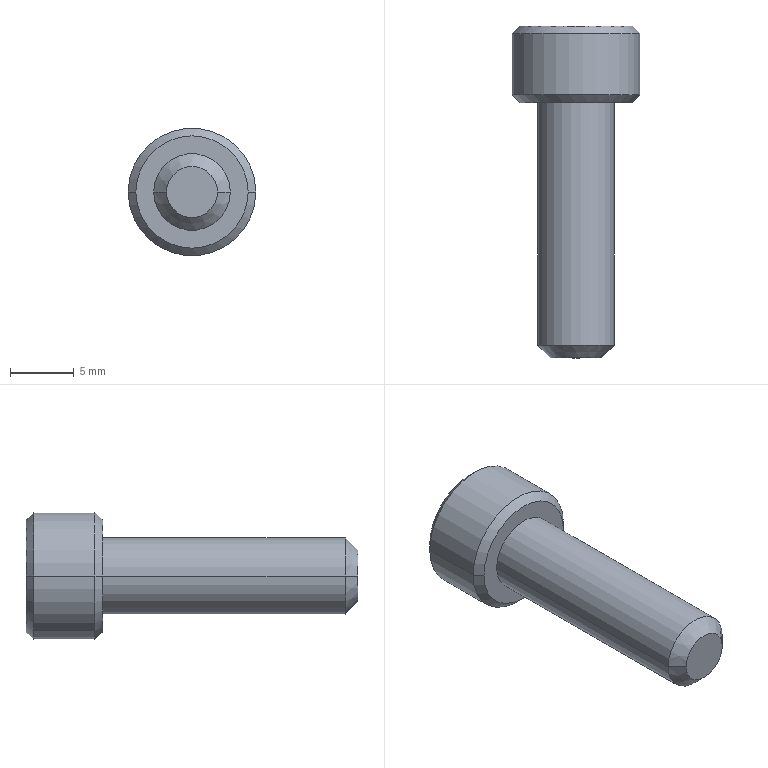Part | STEP file | BB62-M6-20L | 1 solid | 27 faces | box 10 x 26 x 10 mm | volume 939.593 mm3 | plane 15 | cone 8 | cylinder 4 | commonest cylinder face diameters 6 x2 10 x2
STEP:
#1=CARTESIAN_POINT('',(0.,1.349,0.));
#2=VERTEX_POINT('',#1);
#3=CARTESIAN_POINT('',(2.86,3.,0.));
#4=VERTEX_POINT('',#3);
#5=CARTESIAN_POINT('',(0.,1.349,0.));
#6=DIRECTION('',(0.866,0.5,0.));
#7=VECTOR('',#6,1000.);
#8=LINE('',#5,#7);
#9=EDGE_CURVE('',#2,#4,#8,.T.);
#10=ORIENTED_EDGE('',*,*,#9,.F.);
#11=CARTESIAN_POINT('',(-2.86,3.,0.));
#12=VERTEX_POINT('',#11);
#13=CARTESIAN_POINT('',(0.,1.349,0.));
#14=DIRECTION('',(-0.866,0.5,0.));
#15=VECTOR('',#14,1000.);
#16=LINE('',#13,#15);
#17=EDGE_CURVE('',#2,#12,#16,.T.);
#18=ORIENTED_EDGE('',*,*,#17,.T.);
#19=CARTESIAN_POINT('',(-2.477,3.,1.43));
#20=VERTEX_POINT('',#19);
#21=CARTESIAN_POINT('',(0.,3.,0.));
#22=DIRECTION('',(0.,-1.,0.));
#23=DIRECTION('',(-1.,0.,0.));
#24=AXIS2_PLACEMENT_3D('',#21,#22,#23);
#25=CIRCLE('',#24,2.86);
#26=EDGE_CURVE('',#20,#12,#25,.T.);
#27=ORIENTED_EDGE('',*,*,#26,.F.);
#28=CARTESIAN_POINT('',(0.,3.,2.86));
#29=VERTEX_POINT('',#28);
#30=CARTESIAN_POINT('',(0.,3.,0.));
#31=DIRECTION('',(0.,-1.,0.));
#32=DIRECTION('',(-1.,0.,0.));
#33=AXIS2_PLACEMENT_3D('',#30,#31,#32);
#34=CIRCLE('',#33,2.86);
#35=EDGE_CURVE('',#29,#20,#34,.T.);
#36=ORIENTED_EDGE('',*,*,#35,.F.);
#37=CARTESIAN_POINT('',(2.477,3.,1.43));
#38=VERTEX_POINT('',#37);
#39=CARTESIAN_POINT('',(0.,3.,0.));
#40=DIRECTION('',(0.,-1.,0.));
#41=DIRECTION('',(-1.,0.,0.));
#42=AXIS2_PLACEMENT_3D('',#39,#40,#41);
#43=CIRCLE('',#42,2.86);
#44=EDGE_CURVE('',#38,#29,#43,.T.);
#45=ORIENTED_EDGE('',*,*,#44,.F.);
#46=CARTESIAN_POINT('',(0.,3.,0.));
#47=DIRECTION('',(0.,-1.,0.));
#48=DIRECTION('',(-1.,0.,0.));
#49=AXIS2_PLACEMENT_3D('',#46,#47,#48);
#50=CIRCLE('',#49,2.86);
#51=EDGE_CURVE('',#4,#38,#50,.T.);
#52=ORIENTED_EDGE('',*,*,#51,.F.);
#53=EDGE_LOOP('',(#10,#18,#27,#36,#45,#52));
#54=FACE_OUTER_BOUND('',#53,.T.);
#55=CARTESIAN_POINT('',(0.,1001.349,0.));
#56=DIRECTION('',(0.,1.,0.));
#57=DIRECTION('',(1.,0.,0.));
#58=AXIS2_PLACEMENT_3D('',#55,#56,#57);
#59=CONICAL_SURFACE('',#58,1732.051,1.047);
#60=ADVANCED_FACE('',(#54),#59,.F.);
#61=CARTESIAN_POINT('',(2.,-20.,0.));
#62=VERTEX_POINT('',#61);
#63=CARTESIAN_POINT('',(-2.,-20.,0.));
#64=VERTEX_POINT('',#63);
#65=CARTESIAN_POINT('',(0.,-20.,0.));
#66=DIRECTION('',(0.,1.,0.));
#67=DIRECTION('',(1.,0.,0.));
#68=AXIS2_PLACEMENT_3D('',#65,#66,#67);
#69=CIRCLE('',#68,2.);
#70=EDGE_CURVE('',#62,#64,#69,.T.);
#71=ORIENTED_EDGE('',*,*,#70,.T.);
#72=CARTESIAN_POINT('',(-3.,-19.,0.));
#73=VERTEX_POINT('',#72);
#74=CARTESIAN_POINT('',(-2.,-20.,0.));
#75=DIRECTION('',(-0.7071,0.7071,0.));
#76=VECTOR('',#75,1000.);
#77=LINE('',#74,#76);
#78=EDGE_CURVE('',#64,#73,#77,.T.);
#79=ORIENTED_EDGE('',*,*,#78,.T.);
#80=CARTESIAN_POINT('',(3.,-19.,0.));
#81=VERTEX_POINT('',#80);
#82=CARTESIAN_POINT('',(0.,-19.,0.));
#83=DIRECTION('',(0.,-1.,0.));
#84=DIRECTION('',(-1.,0.,0.));
#85=AXIS2_PLACEMENT_3D('',#82,#83,#84);
#86=CIRCLE('',#85,3.);
#87=EDGE_CURVE('',#73,#81,#86,.T.);
#88=ORIENTED_EDGE('',*,*,#87,.T.);
#89=CARTESIAN_POINT('',(2.,-20.,0.));
#90=DIRECTION('',(0.7071,0.7071,0.));
#91=VECTOR('',#90,1000.);
#92=LINE('',#89,#91);
#93=EDGE_CURVE('',#62,#81,#92,.T.);
#94=ORIENTED_EDGE('',*,*,#93,.F.);
#95=EDGE_LOOP('',(#71,#79,#88,#94));
#96=FACE_OUTER_BOUND('',#95,.T.);
#97=CARTESIAN_POINT('',(0.,-20.,0.));
#98=DIRECTION('',(0.,1.,0.));
#99=DIRECTION('',(1.,0.,0.));
#100=AXIS2_PLACEMENT_3D('',#97,#98,#99);
#101=CONICAL_SURFACE('',#100,2.,0.7854);
#102=ADVANCED_FACE('',(#96),#101,.T.);
#103=ORIENTED_EDGE('',*,*,#87,.F.);
#104=CARTESIAN_POINT('',(-3.,0.,0.));
#105=VERTEX_POINT('',#104);
#106=CARTESIAN_POINT('',(-3.,-19.,0.));
#107=DIRECTION('',(0.,1.,0.));
#108=VECTOR('',#107,1000.);
#109=LINE('',#106,#108);
#110=EDGE_CURVE('',#73,#105,#109,.T.);
#111=ORIENTED_EDGE('',*,*,#110,.T.);
#112=CARTESIAN_POINT('',(3.,0.,0.));
#113=VERTEX_POINT('',#112);
#114=CARTESIAN_POINT('',(0.,0.,0.));
#115=DIRECTION('',(0.,-1.,0.));
#116=DIRECTION('',(-1.,0.,0.));
#117=AXIS2_PLACEMENT_3D('',#114,#115,#116);
#118=CIRCLE('',#117,3.);
#119=EDGE_CURVE('',#105,#113,#118,.T.);
#120=ORIENTED_EDGE('',*,*,#119,.T.);
#121=CARTESIAN_POINT('',(3.,-19.,0.));
#122=DIRECTION('',(0.,1.,0.));
#123=VECTOR('',#122,1000.);
#124=LINE('',#121,#123);
#125=EDGE_CURVE('',#81,#113,#124,.T.);
#126=ORIENTED_EDGE('',*,*,#125,.F.);
#127=EDGE_LOOP('',(#103,#111,#120,#126));
#128=FACE_OUTER_BOUND('',#127,.T.);
#129=CARTESIAN_POINT('',(0.,-19.,0.));
#130=DIRECTION('',(0.,1.,0.));
#131=DIRECTION('',(1.,0.,0.));
#132=AXIS2_PLACEMENT_3D('',#129,#130,#131);
#133=CYLINDRICAL_SURFACE('',#132,3.);
#134=ADVANCED_FACE('',(#128),#133,.T.);
#135=CARTESIAN_POINT('',(-4.4,6.,0.));
#136=VERTEX_POINT('',#135);
#137=CARTESIAN_POINT('',(4.4,6.,0.));
#138=VERTEX_POINT('',#137);
#139=CARTESIAN_POINT('',(0.,6.,0.));
#140=DIRECTION('',(0.,-1.,0.));
#141=DIRECTION('',(-1.,0.,0.));
#142=AXIS2_PLACEMENT_3D('',#139,#140,#141);
#143=CIRCLE('',#142,4.4);
#144=EDGE_CURVE('',#136,#138,#143,.T.);
#145=ORIENTED_EDGE('',*,*,#144,.T.);
#146=CARTESIAN_POINT('',(5.,5.4,0.));
#147=VERTEX_POINT('',#146);
#148=CARTESIAN_POINT('',(5.,5.4,0.));
#149=DIRECTION('',(0.7071,-0.7071,0.));
#150=VECTOR('',#149,1000.);
#151=LINE('',#148,#150);
#152=EDGE_CURVE('',#138,#147,#151,.T.);
#153=ORIENTED_EDGE('',*,*,#152,.T.);
#154=CARTESIAN_POINT('',(-5.,5.4,0.));
#155=VERTEX_POINT('',#154);
#156=CARTESIAN_POINT('',(0.,5.4,0.));
#157=DIRECTION('',(0.,-1.,0.));
#158=DIRECTION('',(-1.,0.,0.));
#159=AXIS2_PLACEMENT_3D('',#156,#157,#158);
#160=CIRCLE('',#159,5.);
#161=EDGE_CURVE('',#155,#147,#160,.T.);
#162=ORIENTED_EDGE('',*,*,#161,.F.);
#163=CARTESIAN_POINT('',(-5.,5.4,0.));
#164=DIRECTION('',(-0.7071,-0.7071,0.));
#165=VECTOR('',#164,1000.);
#166=LINE('',#163,#165);
#167=EDGE_CURVE('',#136,#155,#166,.T.);
#168=ORIENTED_EDGE('',*,*,#167,.F.);
#169=EDGE_LOOP('',(#145,#153,#162,#168));
#170=FACE_OUTER_BOUND('',#169,.T.);
#171=CARTESIAN_POINT('',(0.,5.4,0.));
#172=DIRECTION('',(0.,-1.,0.));
#173=DIRECTION('',(-1.,0.,0.));
#174=AXIS2_PLACEMENT_3D('',#171,#172,#173);
#175=CONICAL_SURFACE('',#174,5.,0.7854);
#176=ADVANCED_FACE('',(#170),#175,.T.);
#177=ORIENTED_EDGE('',*,*,#161,.T.);
#178=CARTESIAN_POINT('',(5.,0.6,0.));
#179=VERTEX_POINT('',#178);
#180=CARTESIAN_POINT('',(5.,1.62,0.));
#181=DIRECTION('',(0.,-1.,0.));
#182=VECTOR('',#181,1000.);
#183=LINE('',#180,#182);
#184=EDGE_CURVE('',#147,#179,#183,.T.);
#185=ORIENTED_EDGE('',*,*,#184,.T.);
#186=CARTESIAN_POINT('',(-5.,0.6,0.));
#187=VERTEX_POINT('',#186);
#188=CARTESIAN_POINT('',(0.,0.6,0.));
#189=DIRECTION('',(0.,-1.,0.));
#190=DIRECTION('',(-1.,0.,0.));
#191=AXIS2_PLACEMENT_3D('',#188,#189,#190);
#192=CIRCLE('',#191,5.);
#193=EDGE_CURVE('',#187,#179,#192,.T.);
#194=ORIENTED_EDGE('',*,*,#193,.F.);
#195=CARTESIAN_POINT('',(-5.,1.62,0.));
#196=DIRECTION('',(0.,-1.,0.));
#197=VECTOR('',#196,1000.);
#198=LINE('',#195,#197);
#199=EDGE_CURVE('',#155,#187,#198,.T.);
#200=ORIENTED_EDGE('',*,*,#199,.F.);
#201=EDGE_LOOP('',(#177,#185,#194,#200));
#202=FACE_OUTER_BOUND('',#201,.T.);
#203=CARTESIAN_POINT('',(0.,1.62,0.));
#204=DIRECTION('',(0.,-1.,0.));
#205=DIRECTION('',(-1.,0.,0.));
#206=AXIS2_PLACEMENT_3D('',#203,#204,#205);
#207=CYLINDRICAL_SURFACE('',#206,5.);
#208=ADVANCED_FACE('',(#202),#207,.T.);
#209=CARTESIAN_POINT('',(-4.4,0.,0.));
#210=VERTEX_POINT('',#209);
#211=CARTESIAN_POINT('',(4.4,0.,0.));
#212=VERTEX_POINT('',#211);
#213=CARTESIAN_POINT('',(0.,0.,0.));
#214=DIRECTION('',(0.,-1.,0.));
#215=DIRECTION('',(-1.,0.,0.));
#216=AXIS2_PLACEMENT_3D('',#213,#214,#215);
#217=CIRCLE('',#216,4.4);
#218=EDGE_CURVE('',#210,#212,#217,.T.);
#219=ORIENTED_EDGE('',*,*,#218,.F.);
#220=CARTESIAN_POINT('',(-4.4,0.,0.));
#221=DIRECTION('',(-0.7071,0.7071,0.));
#222=VECTOR('',#221,1000.);
#223=LINE('',#220,#222);
#224=EDGE_CURVE('',#210,#187,#223,.T.);
#225=ORIENTED_EDGE('',*,*,#224,.T.);
#226=ORIENTED_EDGE('',*,*,#193,.T.);
#227=CARTESIAN_POINT('',(4.4,0.,0.));
#228=DIRECTION('',(0.7071,0.7071,0.));
#229=VECTOR('',#228,1000.);
#230=LINE('',#227,#229);
#231=EDGE_CURVE('',#212,#179,#230,.T.);
#232=ORIENTED_EDGE('',*,*,#231,.F.);
#233=EDGE_LOOP('',(#219,#225,#226,#232));
#234=FACE_OUTER_BOUND('',#233,.T.);
#235=CARTESIAN_POINT('',(0.,0.,0.));
#236=DIRECTION('',(0.,1.,0.));
#237=DIRECTION('',(1.,0.,0.));
#238=AXIS2_PLACEMENT_3D('',#235,#236,#237);
#239=CONICAL_SURFACE('',#238,4.4,0.7854);
#240=ADVANCED_FACE('',(#234),#239,.T.);
#241=ORIENTED_EDGE('',*,*,#144,.F.);
#242=CARTESIAN_POINT('',(0.,6.,0.));
#243=DIRECTION('',(0.,-1.,0.));
#244=DIRECTION('',(-1.,0.,0.));
#245=AXIS2_PLACEMENT_3D('',#242,#243,#244);
#246=CIRCLE('',#245,4.4);
#247=EDGE_CURVE('',#138,#136,#246,.T.);
#248=ORIENTED_EDGE('',*,*,#247,.F.);
#249=EDGE_LOOP('',(#241,#248));
#250=FACE_OUTER_BOUND('',#249,.T.);
#251=CARTESIAN_POINT('',(0.,6.,-2.86));
#252=VERTEX_POINT('',#251);
#253=CARTESIAN_POINT('',(-2.477,6.,-1.43));
#254=VERTEX_POINT('',#253);
#255=CARTESIAN_POINT('',(0.,6.,-2.86));
#256=DIRECTION('',(-0.866,0.,0.5));
#257=VECTOR('',#256,1000.);
#258=LINE('',#255,#257);
#259=EDGE_CURVE('',#252,#254,#258,.T.);
#260=ORIENTED_EDGE('',*,*,#259,.F.);
#261=CARTESIAN_POINT('',(2.477,6.,-1.43));
#262=VERTEX_POINT('',#261);
#263=CARTESIAN_POINT('',(2.477,6.,-1.43));
#264=DIRECTION('',(-0.866,0.,-0.5));
#265=VECTOR('',#264,1000.);
#266=LINE('',#263,#265);
#267=EDGE_CURVE('',#262,#252,#266,.T.);
#268=ORIENTED_EDGE('',*,*,#267,.F.);
#269=CARTESIAN_POINT('',(2.477,6.,1.43));
#270=VERTEX_POINT('',#269);
#271=CARTESIAN_POINT('',(2.477,6.,1.43));
#272=DIRECTION('',(0.,0.,-1.));
#273=VECTOR('',#272,1000.);
#274=LINE('',#271,#273);
#275=EDGE_CURVE('',#270,#262,#274,.T.);
#276=ORIENTED_EDGE('',*,*,#275,.F.);
#277=CARTESIAN_POINT('',(0.,6.,2.86));
#278=VERTEX_POINT('',#277);
#279=CARTESIAN_POINT('',(0.,6.,2.86));
#280=DIRECTION('',(0.866,0.,-0.5));
#281=VECTOR('',#280,1000.);
#282=LINE('',#279,#281);
#283=EDGE_CURVE('',#278,#270,#282,.T.);
#284=ORIENTED_EDGE('',*,*,#283,.F.);
#285=CARTESIAN_POINT('',(-2.477,6.,1.43));
#286=VERTEX_POINT('',#285);
#287=CARTESIAN_POINT('',(-2.477,6.,1.43));
#288=DIRECTION('',(0.866,0.,0.5));
#289=VECTOR('',#288,1000.);
#290=LINE('',#287,#289);
#291=EDGE_CURVE('',#286,#278,#290,.T.);
#292=ORIENTED_EDGE('',*,*,#291,.F.);
#293=CARTESIAN_POINT('',(-2.477,6.,-1.43));
#294=DIRECTION('',(0.,0.,1.));
#295=VECTOR('',#294,1000.);
#296=LINE('',#293,#295);
#297=EDGE_CURVE('',#254,#286,#296,.T.);
#298=ORIENTED_EDGE('',*,*,#297,.F.);
#299=EDGE_LOOP('',(#260,#268,#276,#284,#292,#298));
#300=FACE_BOUND('',#299,.T.);
#301=CARTESIAN_POINT('',(4.4,6.,0.));
#302=DIRECTION('',(0.,1.,0.));
#303=DIRECTION('',(1.,0.,0.));
#304=AXIS2_PLACEMENT_3D('',#301,#302,#303);
#305=PLANE('',#304);
#306=ADVANCED_FACE('',(#250,#300),#305,.T.);
#307=CARTESIAN_POINT('',(0.,0.,0.));
#308=DIRECTION('',(0.,-1.,0.));
#309=DIRECTION('',(-1.,0.,0.));
#310=AXIS2_PLACEMENT_3D('',#307,#308,#309);
#311=CIRCLE('',#310,3.);
#312=EDGE_CURVE('',#113,#105,#311,.T.);
#313=ORIENTED_EDGE('',*,*,#312,.F.);
#314=ORIENTED_EDGE('',*,*,#119,.F.);
#315=EDGE_LOOP('',(#313,#314));
#316=FACE_BOUND('',#315,.T.);
#317=CARTESIAN_POINT('',(0.,0.,0.));
#318=DIRECTION('',(0.,-1.,0.));
#319=DIRECTION('',(-1.,0.,0.));
#320=AXIS2_PLACEMENT_3D('',#317,#318,#319);
#321=CIRCLE('',#320,4.4);
#322=EDGE_CURVE('',#212,#210,#321,.T.);
#323=ORIENTED_EDGE('',*,*,#322,.T.);
#324=ORIENTED_EDGE('',*,*,#218,.T.);
#325=EDGE_LOOP('',(#323,#324));
#326=FACE_OUTER_BOUND('',#325,.T.);
#327=CARTESIAN_POINT('',(0.,0.,0.));
#328=DIRECTION('',(0.,-1.,0.));
#329=DIRECTION('',(-1.,0.,0.));
#330=AXIS2_PLACEMENT_3D('',#327,#328,#329);
#331=PLANE('',#330);
#332=ADVANCED_FACE('',(#316,#326),#331,.T.);
#333=ORIENTED_EDGE('',*,*,#224,.F.);
#334=ORIENTED_EDGE('',*,*,#322,.F.);
#335=ORIENTED_EDGE('',*,*,#231,.T.);
#336=CARTESIAN_POINT('',(0.,0.6,0.));
#337=DIRECTION('',(0.,-1.,0.));
#338=DIRECTION('',(-1.,0.,0.));
#339=AXIS2_PLACEMENT_3D('',#336,#337,#338);
#340=CIRCLE('',#339,5.);
#341=EDGE_CURVE('',#179,#187,#340,.T.);
#342=ORIENTED_EDGE('',*,*,#341,.T.);
#343=EDGE_LOOP('',(#333,#334,#335,#342));
#344=FACE_OUTER_BOUND('',#343,.T.);
#345=CARTESIAN_POINT('',(0.,0.,0.));
#346=DIRECTION('',(0.,1.,0.));
#347=DIRECTION('',(1.,0.,0.));
#348=AXIS2_PLACEMENT_3D('',#345,#346,#347);
#349=CONICAL_SURFACE('',#348,4.4,0.7854);
#350=ADVANCED_FACE('',(#344),#349,.T.);
#351=ORIENTED_EDGE('',*,*,#184,.F.);
#352=CARTESIAN_POINT('',(0.,5.4,0.));
#353=DIRECTION('',(0.,-1.,0.));
#354=DIRECTION('',(-1.,0.,0.));
#355=AXIS2_PLACEMENT_3D('',#352,#353,#354);
#356=CIRCLE('',#355,5.);
#357=EDGE_CURVE('',#147,#155,#356,.T.);
#358=ORIENTED_EDGE('',*,*,#357,.T.);
#359=ORIENTED_EDGE('',*,*,#199,.T.);
#360=ORIENTED_EDGE('',*,*,#341,.F.);
#361=EDGE_LOOP('',(#351,#358,#359,#360));
#362=FACE_OUTER_BOUND('',#361,.T.);
#363=CARTESIAN_POINT('',(0.,1.62,0.));
#364=DIRECTION('',(0.,-1.,0.));
#365=DIRECTION('',(-1.,0.,0.));
#366=AXIS2_PLACEMENT_3D('',#363,#364,#365);
#367=CYLINDRICAL_SURFACE('',#366,5.);
#368=ADVANCED_FACE('',(#362),#367,.T.);
#369=ORIENTED_EDGE('',*,*,#152,.F.);
#370=ORIENTED_EDGE('',*,*,#247,.T.);
#371=ORIENTED_EDGE('',*,*,#167,.T.);
#372=ORIENTED_EDGE('',*,*,#357,.F.);
#373=EDGE_LOOP('',(#369,#370,#371,#372));
#374=FACE_OUTER_BOUND('',#373,.T.);
#375=CARTESIAN_POINT('',(0.,5.4,0.));
#376=DIRECTION('',(0.,-1.,0.));
#377=DIRECTION('',(-1.,0.,0.));
#378=AXIS2_PLACEMENT_3D('',#375,#376,#377);
#379=CONICAL_SURFACE('',#378,5.,0.7854);
#380=ADVANCED_FACE('',(#374),#379,.T.);
#381=ORIENTED_EDGE('',*,*,#110,.F.);
#382=CARTESIAN_POINT('',(0.,-19.,0.));
#383=DIRECTION('',(0.,-1.,0.));
#384=DIRECTION('',(-1.,0.,0.));
#385=AXIS2_PLACEMENT_3D('',#382,#383,#384);
#386=CIRCLE('',#385,3.);
#387=EDGE_CURVE('',#81,#73,#386,.T.);
#388=ORIENTED_EDGE('',*,*,#387,.F.);
#389=ORIENTED_EDGE('',*,*,#125,.T.);
#390=ORIENTED_EDGE('',*,*,#312,.T.);
#391=EDGE_LOOP('',(#381,#388,#389,#390));
#392=FACE_OUTER_BOUND('',#391,.T.);
#393=CARTESIAN_POINT('',(0.,-19.,0.));
#394=DIRECTION('',(0.,1.,0.));
#395=DIRECTION('',(1.,0.,0.));
#396=AXIS2_PLACEMENT_3D('',#393,#394,#395);
#397=CYLINDRICAL_SURFACE('',#396,3.);
#398=ADVANCED_FACE('',(#392),#397,.T.);
#399=ORIENTED_EDGE('',*,*,#70,.F.);
#400=CARTESIAN_POINT('',(0.,-20.,0.));
#401=DIRECTION('',(0.,1.,0.));
#402=DIRECTION('',(1.,0.,0.));
#403=AXIS2_PLACEMENT_3D('',#400,#401,#402);
#404=CIRCLE('',#403,2.);
#405=EDGE_CURVE('',#64,#62,#404,.T.);
#406=ORIENTED_EDGE('',*,*,#405,.F.);
#407=EDGE_LOOP('',(#399,#406));
#408=FACE_OUTER_BOUND('',#407,.T.);
#409=CARTESIAN_POINT('',(0.,-20.,0.));
#410=DIRECTION('',(0.,-1.,0.));
#411=DIRECTION('',(-1.,0.,0.));
#412=AXIS2_PLACEMENT_3D('',#409,#410,#411);
#413=PLANE('',#412);
#414=ADVANCED_FACE('',(#408),#413,.T.);
#415=ORIENTED_EDGE('',*,*,#78,.F.);
#416=ORIENTED_EDGE('',*,*,#405,.T.);
#417=ORIENTED_EDGE('',*,*,#93,.T.);
#418=ORIENTED_EDGE('',*,*,#387,.T.);
#419=EDGE_LOOP('',(#415,#416,#417,#418));
#420=FACE_OUTER_BOUND('',#419,.T.);
#421=CARTESIAN_POINT('',(0.,-20.,0.));
#422=DIRECTION('',(0.,1.,0.));
#423=DIRECTION('',(1.,0.,0.));
#424=AXIS2_PLACEMENT_3D('',#421,#422,#423);
#425=CONICAL_SURFACE('',#424,2.,0.7854);
#426=ADVANCED_FACE('',(#420),#425,.T.);
#427=CARTESIAN_POINT('',(2.477,3.,-1.43));
#428=VERTEX_POINT('',#427);
#429=CARTESIAN_POINT('',(0.,3.,-2.86));
#430=VERTEX_POINT('',#429);
#431=CARTESIAN_POINT('',(2.477,3.,-1.43));
#432=DIRECTION('',(-0.866,0.,-0.5));
#433=VECTOR('',#432,1000.);
#434=LINE('',#431,#433);
#435=EDGE_CURVE('',#428,#430,#434,.T.);
#436=ORIENTED_EDGE('',*,*,#435,.F.);
#437=CARTESIAN_POINT('',(2.477,6.,-1.43));
#438=DIRECTION('',(0.,-1.,0.));
#439=VECTOR('',#438,1000.);
#440=LINE('',#437,#439);
#441=EDGE_CURVE('',#262,#428,#440,.T.);
#442=ORIENTED_EDGE('',*,*,#441,.F.);
#443=ORIENTED_EDGE('',*,*,#267,.T.);
#444=CARTESIAN_POINT('',(0.,6.,-2.86));
#445=DIRECTION('',(0.,-1.,0.));
#446=VECTOR('',#445,1000.);
#447=LINE('',#444,#446);
#448=EDGE_CURVE('',#252,#430,#447,.T.);
#449=ORIENTED_EDGE('',*,*,#448,.T.);
#450=EDGE_LOOP('',(#436,#442,#443,#449));
#451=FACE_OUTER_BOUND('',#450,.T.);
#452=CARTESIAN_POINT('',(2.477,6.,-1.43));
#453=DIRECTION('',(-0.5,0.,0.866));
#454=DIRECTION('',(0.866,0.,0.5));
#455=AXIS2_PLACEMENT_3D('',#452,#453,#454);
#456=PLANE('',#455);
#457=ADVANCED_FACE('',(#451),#456,.T.);
#458=CARTESIAN_POINT('',(-2.477,3.,-1.43));
#459=VERTEX_POINT('',#458);
#460=CARTESIAN_POINT('',(0.,3.,-2.86));
#461=DIRECTION('',(-0.866,0.,0.5));
#462=VECTOR('',#461,1000.);
#463=LINE('',#460,#462);
#464=EDGE_CURVE('',#430,#459,#463,.T.);
#465=ORIENTED_EDGE('',*,*,#464,.F.);
#466=ORIENTED_EDGE('',*,*,#448,.F.);
#467=ORIENTED_EDGE('',*,*,#259,.T.);
#468=CARTESIAN_POINT('',(-2.477,6.,-1.43));
#469=DIRECTION('',(0.,-1.,0.));
#470=VECTOR('',#469,1000.);
#471=LINE('',#468,#470);
#472=EDGE_CURVE('',#254,#459,#471,.T.);
#473=ORIENTED_EDGE('',*,*,#472,.T.);
#474=EDGE_LOOP('',(#465,#466,#467,#473));
#475=FACE_OUTER_BOUND('',#474,.T.);
#476=CARTESIAN_POINT('',(0.,6.,-2.86));
#477=DIRECTION('',(0.5,0.,0.866));
#478=DIRECTION('',(0.866,0.,-0.5));
#479=AXIS2_PLACEMENT_3D('',#476,#477,#478);
#480=PLANE('',#479);
#481=ADVANCED_FACE('',(#475),#480,.T.);
#482=CARTESIAN_POINT('',(-2.477,3.,-1.43));
#483=DIRECTION('',(0.,0.,1.));
#484=VECTOR('',#483,1000.);
#485=LINE('',#482,#484);
#486=EDGE_CURVE('',#459,#20,#485,.T.);
#487=ORIENTED_EDGE('',*,*,#486,.F.);
#488=ORIENTED_EDGE('',*,*,#472,.F.);
#489=ORIENTED_EDGE('',*,*,#297,.T.);
#490=CARTESIAN_POINT('',(-2.477,6.,1.43));
#491=DIRECTION('',(0.,-1.,0.));
#492=VECTOR('',#491,1000.);
#493=LINE('',#490,#492);
#494=EDGE_CURVE('',#286,#20,#493,.T.);
#495=ORIENTED_EDGE('',*,*,#494,.T.);
#496=EDGE_LOOP('',(#487,#488,#489,#495));
#497=FACE_OUTER_BOUND('',#496,.T.);
#498=CARTESIAN_POINT('',(-2.477,6.,-1.43));
#499=DIRECTION('',(1.,0.,0.));
#500=DIRECTION('',(0.,0.,-1.));
#501=AXIS2_PLACEMENT_3D('',#498,#499,#500);
#502=PLANE('',#501);
#503=ADVANCED_FACE('',(#497),#502,.T.);
#504=CARTESIAN_POINT('',(-2.477,3.,1.43));
#505=DIRECTION('',(0.866,0.,0.5));
#506=VECTOR('',#505,1000.);
#507=LINE('',#504,#506);
#508=EDGE_CURVE('',#20,#29,#507,.T.);
#509=ORIENTED_EDGE('',*,*,#508,.F.);
#510=ORIENTED_EDGE('',*,*,#494,.F.);
#511=ORIENTED_EDGE('',*,*,#291,.T.);
#512=CARTESIAN_POINT('',(0.,6.,2.86));
#513=DIRECTION('',(0.,-1.,0.));
#514=VECTOR('',#513,1000.);
#515=LINE('',#512,#514);
#516=EDGE_CURVE('',#278,#29,#515,.T.);
#517=ORIENTED_EDGE('',*,*,#516,.T.);
#518=EDGE_LOOP('',(#509,#510,#511,#517));
#519=FACE_OUTER_BOUND('',#518,.T.);
#520=CARTESIAN_POINT('',(-2.477,6.,1.43));
#521=DIRECTION('',(0.5,0.,-0.866));
#522=DIRECTION('',(-0.866,0.,-0.5));
#523=AXIS2_PLACEMENT_3D('',#520,#521,#522);
#524=PLANE('',#523);
#525=ADVANCED_FACE('',(#519),#524,.T.);
#526=CARTESIAN_POINT('',(0.,3.,2.86));
#527=DIRECTION('',(0.866,0.,-0.5));
#528=VECTOR('',#527,1000.);
#529=LINE('',#526,#528);
#530=EDGE_CURVE('',#29,#38,#529,.T.);
#531=ORIENTED_EDGE('',*,*,#530,.F.);
#532=ORIENTED_EDGE('',*,*,#516,.F.);
#533=ORIENTED_EDGE('',*,*,#283,.T.);
#534=CARTESIAN_POINT('',(2.477,6.,1.43));
#535=DIRECTION('',(0.,-1.,0.));
#536=VECTOR('',#535,1000.);
#537=LINE('',#534,#536);
#538=EDGE_CURVE('',#270,#38,#537,.T.);
#539=ORIENTED_EDGE('',*,*,#538,.T.);
#540=EDGE_LOOP('',(#531,#532,#533,#539));
#541=FACE_OUTER_BOUND('',#540,.T.);
#542=CARTESIAN_POINT('',(0.,6.,2.86));
#543=DIRECTION('',(-0.5,0.,-0.866));
#544=DIRECTION('',(-0.866,0.,0.5));
#545=AXIS2_PLACEMENT_3D('',#542,#543,#544);
#546=PLANE('',#545);
#547=ADVANCED_FACE('',(#541),#546,.T.);
#548=CARTESIAN_POINT('',(2.477,3.,1.43));
#549=DIRECTION('',(0.,0.,-1.));
#550=VECTOR('',#549,1000.);
#551=LINE('',#548,#550);
#552=EDGE_CURVE('',#38,#428,#551,.T.);
#553=ORIENTED_EDGE('',*,*,#552,.F.);
#554=ORIENTED_EDGE('',*,*,#538,.F.);
#555=ORIENTED_EDGE('',*,*,#275,.T.);
#556=ORIENTED_EDGE('',*,*,#441,.T.);
#557=EDGE_LOOP('',(#553,#554,#555,#556));
#558=FACE_OUTER_BOUND('',#557,.T.);
#559=CARTESIAN_POINT('',(2.477,6.,1.43));
#560=DIRECTION('',(-1.,0.,0.));
#561=DIRECTION('',(0.,0.,1.));
#562=AXIS2_PLACEMENT_3D('',#559,#560,#561);
#563=PLANE('',#562);
#564=ADVANCED_FACE('',(#558),#563,.T.);
#565=ORIENTED_EDGE('',*,*,#435,.T.);
#566=CARTESIAN_POINT('',(0.,3.,0.));
#567=DIRECTION('',(0.,-1.,0.));
#568=DIRECTION('',(-1.,0.,0.));
#569=AXIS2_PLACEMENT_3D('',#566,#567,#568);
#570=CIRCLE('',#569,2.86);
#571=EDGE_CURVE('',#430,#428,#570,.T.);
#572=ORIENTED_EDGE('',*,*,#571,.T.);
#573=EDGE_LOOP('',(#565,#572));
#574=FACE_OUTER_BOUND('',#573,.T.);
#575=CARTESIAN_POINT('',(0.,3.,0.));
#576=DIRECTION('',(0.,1.,0.));
#577=DIRECTION('',(1.,0.,0.));
#578=AXIS2_PLACEMENT_3D('',#575,#576,#577);
#579=PLANE('',#578);
#580=ADVANCED_FACE('',(#574),#579,.F.);
#581=ORIENTED_EDGE('',*,*,#552,.T.);
#582=CARTESIAN_POINT('',(0.,3.,0.));
#583=DIRECTION('',(0.,-1.,0.));
#584=DIRECTION('',(-1.,0.,0.));
#585=AXIS2_PLACEMENT_3D('',#582,#583,#584);
#586=CIRCLE('',#585,2.86);
#587=EDGE_CURVE('',#428,#4,#586,.T.);
#588=ORIENTED_EDGE('',*,*,#587,.T.);
#589=ORIENTED_EDGE('',*,*,#51,.T.);
#590=EDGE_LOOP('',(#581,#588,#589));
#591=FACE_OUTER_BOUND('',#590,.T.);
#592=CARTESIAN_POINT('',(0.,3.,0.));
#593=DIRECTION('',(0.,1.,0.));
#594=DIRECTION('',(1.,0.,0.));
#595=AXIS2_PLACEMENT_3D('',#592,#593,#594);
#596=PLANE('',#595);
#597=ADVANCED_FACE('',(#591),#596,.F.);
#598=ORIENTED_EDGE('',*,*,#530,.T.);
#599=ORIENTED_EDGE('',*,*,#44,.T.);
#600=EDGE_LOOP('',(#598,#599));
#601=FACE_OUTER_BOUND('',#600,.T.);
#602=CARTESIAN_POINT('',(0.,3.,0.));
#603=DIRECTION('',(0.,1.,0.));
#604=DIRECTION('',(1.,0.,0.));
#605=AXIS2_PLACEMENT_3D('',#602,#603,#604);
#606=PLANE('',#605);
#607=ADVANCED_FACE('',(#601),#606,.F.);
#608=ORIENTED_EDGE('',*,*,#508,.T.);
#609=ORIENTED_EDGE('',*,*,#35,.T.);
#610=EDGE_LOOP('',(#608,#609));
#611=FACE_OUTER_BOUND('',#610,.T.);
#612=CARTESIAN_POINT('',(0.,3.,0.));
#613=DIRECTION('',(0.,1.,0.));
#614=DIRECTION('',(1.,0.,0.));
#615=AXIS2_PLACEMENT_3D('',#612,#613,#614);
#616=PLANE('',#615);
#617=ADVANCED_FACE('',(#611),#616,.F.);
#618=ORIENTED_EDGE('',*,*,#486,.T.);
#619=ORIENTED_EDGE('',*,*,#26,.T.);
#620=CARTESIAN_POINT('',(0.,3.,0.));
#621=DIRECTION('',(0.,-1.,0.));
#622=DIRECTION('',(-1.,0.,0.));
#623=AXIS2_PLACEMENT_3D('',#620,#621,#622);
#624=CIRCLE('',#623,2.86);
#625=EDGE_CURVE('',#12,#459,#624,.T.);
#626=ORIENTED_EDGE('',*,*,#625,.T.);
#627=EDGE_LOOP('',(#618,#619,#626));
#628=FACE_OUTER_BOUND('',#627,.T.);
#629=CARTESIAN_POINT('',(0.,3.,0.));
#630=DIRECTION('',(0.,1.,0.));
#631=DIRECTION('',(1.,0.,0.));
#632=AXIS2_PLACEMENT_3D('',#629,#630,#631);
#633=PLANE('',#632);
#634=ADVANCED_FACE('',(#628),#633,.F.);
#635=ORIENTED_EDGE('',*,*,#464,.T.);
#636=CARTESIAN_POINT('',(0.,3.,0.));
#637=DIRECTION('',(0.,-1.,0.));
#638=DIRECTION('',(-1.,0.,0.));
#639=AXIS2_PLACEMENT_3D('',#636,#637,#638);
#640=CIRCLE('',#639,2.86);
#641=EDGE_CURVE('',#459,#430,#640,.T.);
#642=ORIENTED_EDGE('',*,*,#641,.T.);
#643=EDGE_LOOP('',(#635,#642));
#644=FACE_OUTER_BOUND('',#643,.T.);
#645=CARTESIAN_POINT('',(0.,3.,0.));
#646=DIRECTION('',(0.,1.,0.));
#647=DIRECTION('',(1.,0.,0.));
#648=AXIS2_PLACEMENT_3D('',#645,#646,#647);
#649=PLANE('',#648);
#650=ADVANCED_FACE('',(#644),#649,.F.);
#651=ORIENTED_EDGE('',*,*,#17,.F.);
#652=ORIENTED_EDGE('',*,*,#9,.T.);
#653=ORIENTED_EDGE('',*,*,#587,.F.);
#654=ORIENTED_EDGE('',*,*,#571,.F.);
#655=ORIENTED_EDGE('',*,*,#641,.F.);
#656=ORIENTED_EDGE('',*,*,#625,.F.);
#657=EDGE_LOOP('',(#651,#652,#653,#654,#655,#656));
#658=FACE_OUTER_BOUND('',#657,.T.);
#659=CARTESIAN_POINT('',(0.,1001.349,0.));
#660=DIRECTION('',(0.,1.,0.));
#661=DIRECTION('',(1.,0.,0.));
#662=AXIS2_PLACEMENT_3D('',#659,#660,#661);
#663=CONICAL_SURFACE('',#662,1732.051,1.047);
#664=ADVANCED_FACE('',(#658),#663,.F.);
#665=CLOSED_SHELL('',(#60,#102,#134,#176,#208,#240,#306,#332,#350,#368,#380,#398,#414,#426,#457,#481,#503,#525,#547,#564,#580,#597,#607,#617,#634,#650,#664));
#666=MANIFOLD_SOLID_BREP('',#665);
#667=CARTESIAN_POINT('',(0.,0.,0.));
#668=DIRECTION('',(0.,0.,1.));
#669=DIRECTION('',(1.,0.,0.));
#670=AXIS2_PLACEMENT_3D('',#667,#668,#669);
#671=(LENGTH_UNIT()NAMED_UNIT(*)SI_UNIT(.MILLI.,.METRE.));
#672=UNCERTAINTY_MEASURE_WITH_UNIT(LENGTH_MEASURE(0.00001),#671,'','');
#673=(NAMED_UNIT(*)PLANE_ANGLE_UNIT()SI_UNIT($,.RADIAN.));
#674=(NAMED_UNIT(*)SI_UNIT($,.STERADIAN.)SOLID_ANGLE_UNIT());
#675=(GEOMETRIC_REPRESENTATION_CONTEXT(3)GLOBAL_UNCERTAINTY_ASSIGNED_CONTEXT((#672))GLOBAL_UNIT_ASSIGNED_CONTEXT((#671,#673,#674))REPRESENTATION_CONTEXT('',''));
#676=ADVANCED_BREP_SHAPE_REPRESENTATION('',(#666,#670),#675);